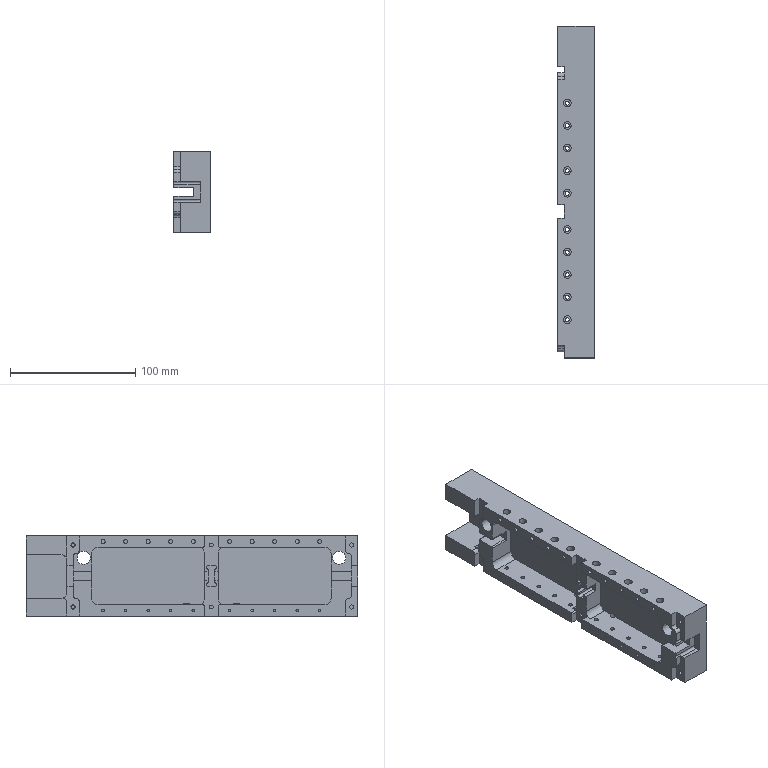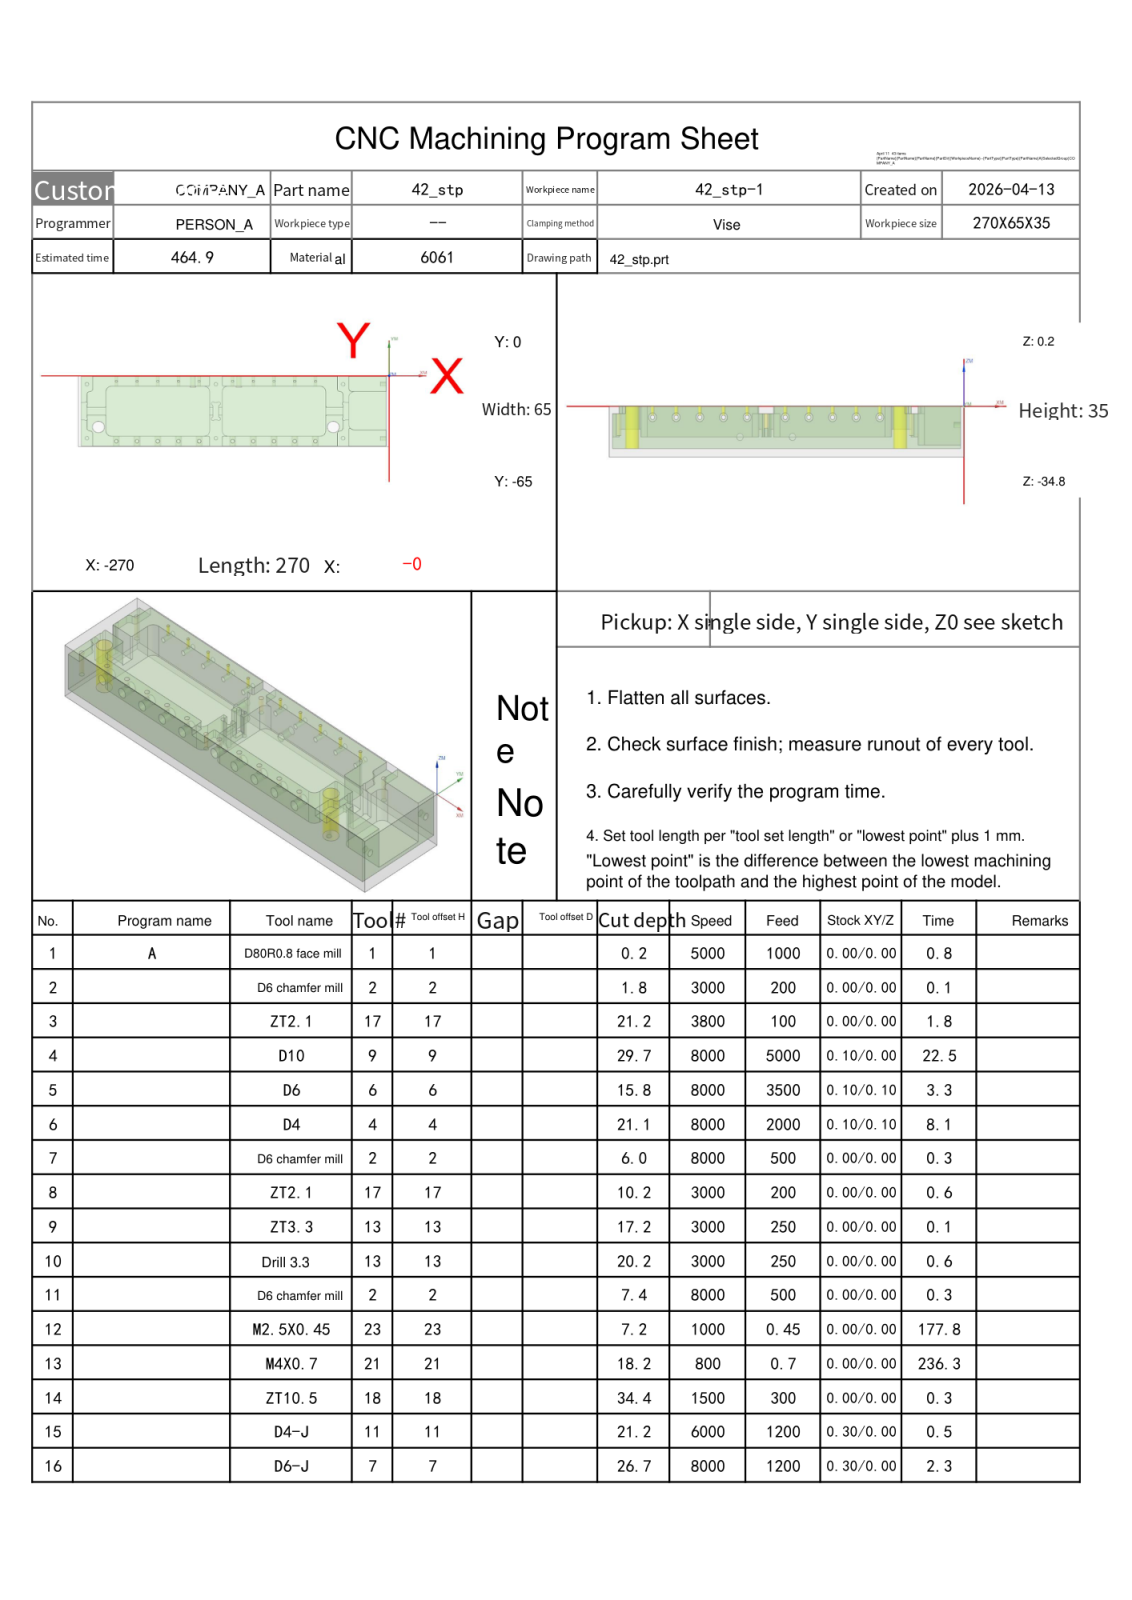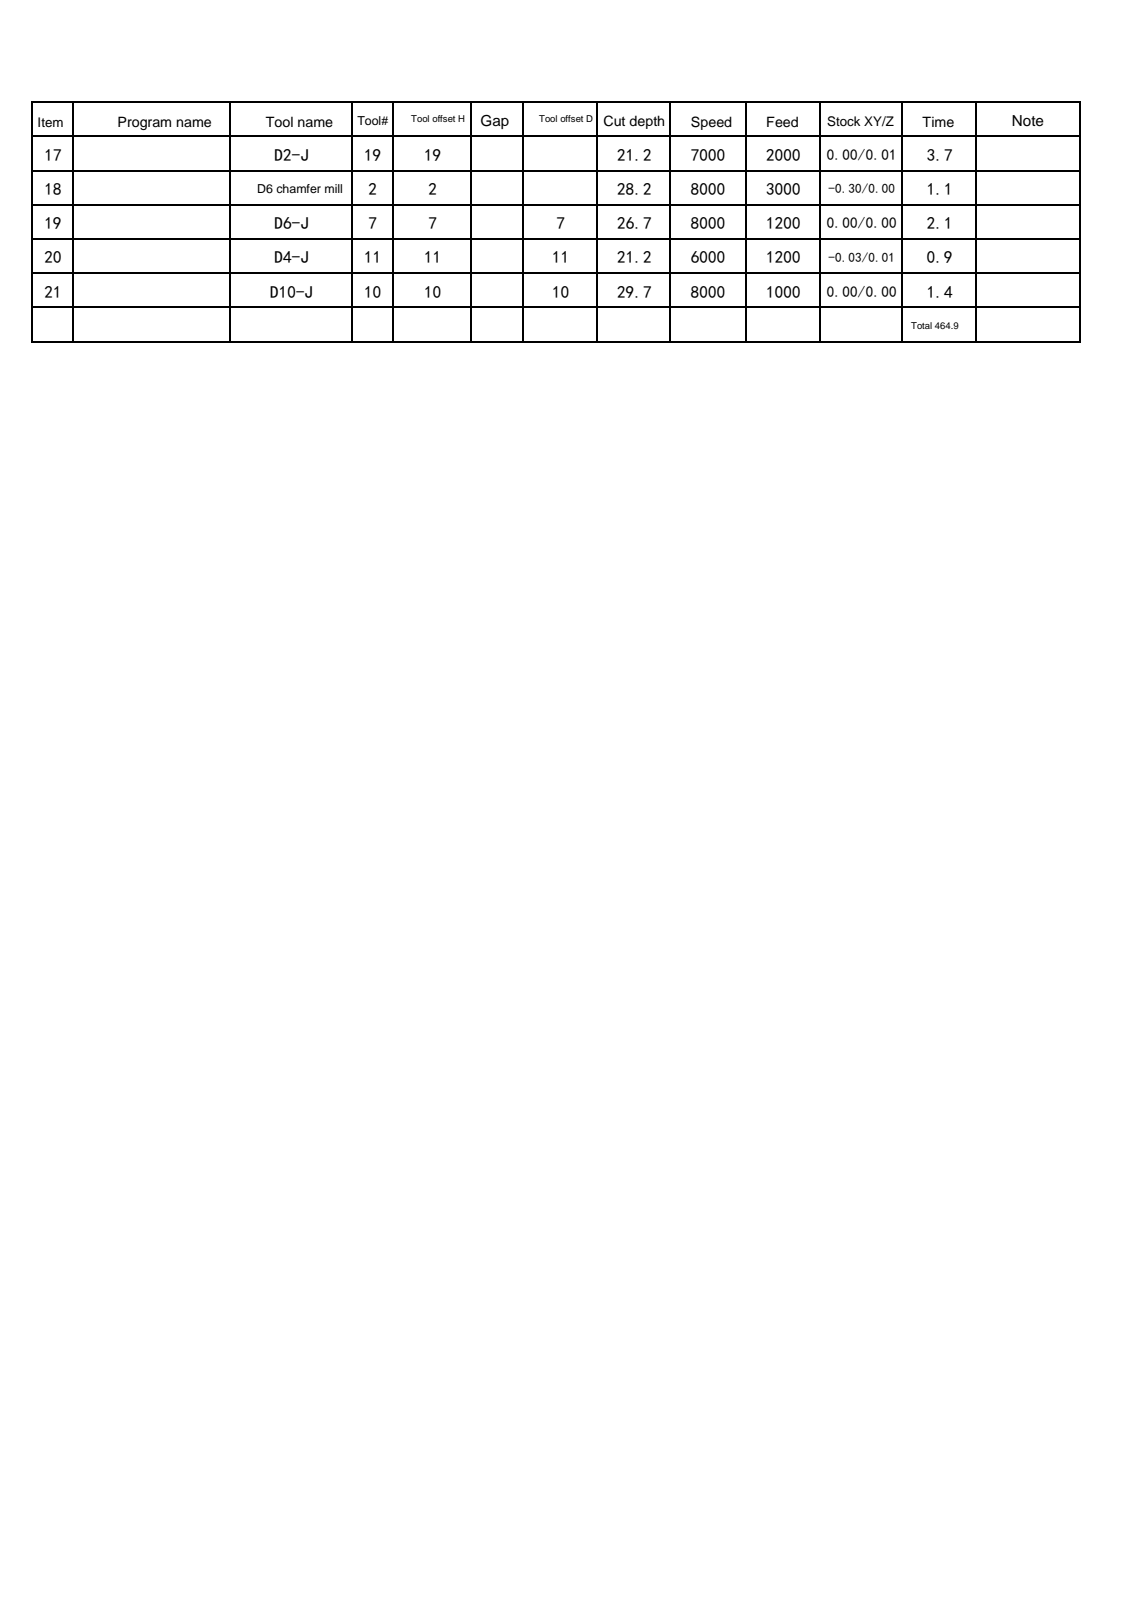NC program | NX | posted by the shop | part box 29 x 265 x 64 mm
Lines 11165 to 11782 of 41846:
N7 T02 M06
(D6 chamfer mill  D=6. R=0. H=02 ce=0.00 di=0.10)
G00 G90 G54 X-48.5 Y-47. M03 S8000
G43 H02 Z20.
M08
G98 G82 X-48.5 Y-47. Z-.8 R1. F500.
X-252.5
G80
G00 Z20.
G00 G90 X-40. Y-7.75 M03 S8000
Z20.
G98 G81 X-40. Y-7.75 Z-5.8 R-4. F500.
X-64. Y-5. Z-.8 R1.
X-82.
X-100.
X-118.
X-136.
X-150.5 Y-7.75 Z-5.8 R-4.
X-165. Y-5. Z-.8 R1.
X-183.
X-201.
X-219.
X-237.
X-262.5 Y-7.75 Z-5.8 R-4.
Y-57.25
X-237. Y-60. Z-.8 R1.
X-219.
X-201.
X-183.
X-165.
X-150.5 Y-57.25 Z-5.8 R-4.
X-136. Y-60. Z-.8 R1.
X-118.
X-100.
X-82.
X-64.
X-40. Y-57.25 Z-5.8 R-4.
G80
G00 Z20.
G00 G90 X-262.5 Y-7.75 M03 S8000
Z20.
G98 G81 X-262.5 Y-7.75 Z-5.8 R-4. F500.
X-237. Y-5. Z-.8 R1.
X-219.
X-201.
X-183.
X-165.
X-150.5 Y-7.75 Z-5.8 R-4.
X-136. Y-5. Z-.8 R1.
X-118.
X-100.
X-82.
X-64.
X-40. Y-7.75 Z-5.8 R-4.
Y-57.25
X-64. Y-60. Z-.8 R1.
X-82.
X-100.
X-118.
X-136.
X-150.5 Y-57.25 Z-5.8 R-4.
X-165. Y-60. Z-.8 R1.
X-183.
X-201.
X-219.
X-237.
X-262.5 Y-57.25 Z-5.8 R-4.
G80
G00 Z20.
G91 G28 Z0.0
M05
M09
G91 G28 Z0.0
M01
N8 T17 M06
(ZT2.1 D=2.1 DR_a=118 H=17)
G00 G90 G54 X-237. Y-5. M03 S3000
G43 H17 Z20.
M08
G98 G83 X-237. Y-5. Z-10. R1. F200. Q2.
X-219.
X-201.
X-183.
X-165.
X-136.
X-118.
X-100.
X-82.
X-64.
G80
G00 Z20.
G91 G28 Z0.0
M05
M09
G91 G28 Z0.0
M01
N9 T13 M06
(ZT3.3 D=3.3 DR_a=118 H=13)
G00 G90 G54 X-150.5 Y-7.75 M03 S3000
G43 H13 Z20.
M08
G98 G83 X-150.5 Y-7.75 Z-17. R-4. F250. Q2.
Y-57.25
G80
G00 Z20.
G91 G28 Z0.0
M05
M09
G91 G28 Z0.0
M01
N10 T13 M06
(Drill 3.3 D=3.3 DR_a=118 H=13)
G00 G90 G54 X-262.5 Y-7.75 M03 S3000
G43 H13 Z20.
M08
G98 G83 X-262.5 Y-7.75 Z-20. R-4. F250. Q2.
Y-57.25
G98 G83 X-237. Y-60. Z-6.926 R1. Q2.
X-219.
X-201.
X-183.
X-165.
X-136.
X-118.
X-100.
X-82.
X-64.
G98 G83 X-40. Y-57.25 Z-20. R-4. Q2.
Y-7.75
G80
G00 Z20.
G91 G28 Z0.0
M05
M09
G91 G28 Z0.0
M01
N11 T02 M06
(D6 chamfer mill  D=6. R=0. H=02 ce=0.00 di=0.10)
G00 G90 G54 X-237. Y-5. M03 S8000
G43 H02 Z20.
M08
G98 G81 X-237. Y-5. Z-1.5 R3. F500.
X-219.
X-201.
X-183.
X-165.
X-136.
X-118.
X-100.
X-82.
X-64.
G80
G00 Z20.
G00 G90 X-150.5 Y-7.75 M03 S8000
Z20.
G98 G81 X-150.5 Y-7.75 Z-7.15 R-2. F500.
Y-57.25
G80
G00 Z20.
G00 G90 X-262.5 Y-7.75 M03 S8000
Z20.
G98 G81 X-262.5 Y-7.75 Z-7.2 R-2. F500.
Y-57.25
X-237. Y-60. Z-2.2 R3.
X-219.
X-201.
X-183.
X-165.
X-136.
X-118.
X-100.
X-82.
X-64.
X-40. Y-57.25 Z-7.2 R-2.
Y-7.75
G80
G00 Z20.
G91 G28 Z0.0
M05
M09
G91 G28 Z0.0
M01
N12 T23 M06
(M2.5X0.45 D=2.05 DR_a=180 H=23)
G00 G90 G54 X-237. Y-5. M03 S1000
G43 H23 Z20.
M08
G95
G98 G84 X-237. Y-5. Z-7. R1. F.45 Q2.
X-219.
X-201.
X-183.
X-165.
X-136.
X-118.
X-100.
X-82.
X-64.
G80
G94
G00 Z20.
G91 G28 Z0.0
M05
M09
G91 G28 Z0.0
M01
N13 T21 M06
(M4X0.7 D=3.3 DR_a=180 H=21)
G00 G90 G54 X-262.5 Y-57.25 M03 S800
G43 H21 Z20.
M08
G95
G98 G84 X-262.5 Y-57.25 Z-18. R1. F.7 Q4.
G98 G84 X-237. Y-60. Z-5.935 R1.
X-219.
X-201.
X-183.
X-165.
X-136.
X-118.
X-100.
X-82.
X-64.
G98 G84 X-40. Y-57.25 Z-18. R1.
Y-7.75
X-262.5
G80
G94
G00 Z20.
G00 G90 X-150.5 Y-57.25 M03 S800
Z20.
G95
G98 G84 X-150.5 Y-57.25 Z-14. R-4. F.7 Q4.
Y-7.75
G80
G94
G00 Z20.
G91 G28 Z0.0
M05
M09
G91 G28 Z0.0
M01
N14 T18 M06
(ZT10.5 D=10.5 DR_a=118 H=18)
G00 G90 G54 X-48.5 Y-47. M03 S1500
G43 H18 Z20.
M08
G98 G83 X-48.5 Y-47. Z-34.155 R1. F300. Q3.
X-252.5
G80
G00 Z20.
G91 G28 Z0.0
M05
M09
G91 G28 Z0.0
M01
N15 T11 M06
(D4-J  D=4. R=0. H=11 ce=0.30 di=0.00)
G00 G90 G54 X-30. Y-32.5 M03 S6000
G43 H11 Z20.
M08
Z-20.5
G01 Z-21. F1200.
X-34.6
Y-38.2
X-37.7
Y-26.8
X-34.6
Y-32.5
Y-33.
X-30.
Z-20.5
G00 Z20.
X-272.5 Y-32.5
Z-20.5
G01 Z-21.
X-267.9
Y-26.8
X-264.8
Y-38.2
X-267.9
Y-32.5
Y-32.
X-272.5
Z-20.5
G00 Z20.
G00 G90 X-40. Y-69.8 M03 S6000
Z20.
Z-4.5
G01 Z-5. F1200.
Y-64.9
X-42.7
Y-53.
G02 X-42.5 Y-52.8 I.2 J0.0
G03 X-37.7 Y-48. I0.0 J4.8
G01 Y-40.618
G03 X-37.759 Y-40.1 I-2.3 J0.0
G01 X-34.6
Y-44.75
G03 X-34.44 Y-45.952 I4.6 J0.0
X-37.3 Y-49.222 I.44 J-3.27
G01 Y-64.9
X-40.
Y-63.1
X-40.9
Y-54.403
G03 X-39.1 Y-53.657 I-1.6 J6.403
G01 Y-63.1
X-40.
X-40.5
Y-69.8
Z-4.5
G00 Z20.
G00 G90 X-40. Y4.8 M03 S6000
Z20.
Z-4.5
G01 Z-5. F1200.
Y-.1
X-37.3
Y-11.5
G03 X-33.546 Y-16.57 I5.3 J0.0
X-34.6 Y-19.5 I3.546 J-2.93
G01 Y-24.9
X-37.759
G03 X-37.7 Y-24.382 I-2.241 J.518
G01 Y-17.
G03 X-42.5 Y-12.2 I-4.8 J0.0
G02 X-42.7 Y-12. I0.0 J.2
G01 Y-.1
X-40.
Y-1.9
X-39.1
Y-11.343
G03 X-40.9 Y-10.597 I-3.4 J-5.657
G01 Y-1.9
X-40.
X-39.5
Y4.8
Z-4.5
G00 Z20.
G00 G90 X-272.5 Y-57.867 M03 S6000
Z20.
Z-4.5
G01 Z-5. F1200.
X-267.9
Y-40.1
X-264.741
G03 X-264.8 Y-40.618 I2.241 J-.518
G01 Y-48.
G03 X-260. Y-52.8 I4.8 J0.0
G02 X-259.8 Y-53. I0.0 J-.2
G01 Y-64.9
X-267.9
Y-57.867
X-265.1
Y-53.635
X-265.831 Y-51.636
X-265.1 Y-53.635
G03 X-262.6 Y-55.141 I5.1 J5.635
G01 Y-62.1
X-265.1
Y-57.867
Y-57.367
X-272.5
Z-4.5
G00 Z20.
Y-7.133
Z-4.5
G01 Z-5.
X-267.9
Y-.1
X-259.8
Y-12.
G02 X-260. Y-12.2 I-.2 J0.0
G03 X-264.8 Y-17. I0.0 J-4.8
G01 Y-24.382
G03 X-264.741 Y-24.9 I2.3 J0.0
G01 X-267.9
Y-7.133
X-265.1
Y-2.9
X-262.6
Y-9.859
G03 X-265.1 Y-11.365 I2.6 J-7.141
G01 X-265.831 Y-13.364
X-265.1 Y-11.365
Y-7.133
Y-6.633
X-272.5
Z-4.5
G00 Z20.
G91 G28 Z0.0
M05
M09
G91 G28 Z0.0
M01
N16 T07 M06
(D6-J  D=6. R=0. H=07 ce=0.30 di=0.00)
G00 G90 G54 X-242.7 Y-14.776 M03 S6000
G43 H07 Z20.
M08
Z-19.5
G01 Y-14.315 Z-19.516 F1200.
X-242.589 Y-13.867 Z-19.532
X-242.361 Y-13.465 Z-19.548
X-242.035 Y-13.139 Z-19.564
X-241.633 Y-12.911 Z-19.581
X-241.185 Y-12.8 Z-19.597
X-201. Z-21.
X-161.
G02 X-159.3 Y-14.5 I0.0 J-1.7
G01 Y-50.5
G02 X-161. Y-52.2 I-1.7 J0.0
G01 X-241.
G02 X-242.7 Y-50.5 I0.0 J1.7
G01 Y-14.5
G02 X-241. Y-12.8 I1.7 J0.0
G01 X-201.
Y-17.
X-163.5
Y-48.
X-238.5
Y-17.
X-201.
Y-21.2
X-167.7
Y-43.8
X-234.3
Y-21.2
X-201.
Y-25.4
X-171.9
Y-39.6
X-230.1
Y-25.4
X-201.
Y-29.6
X-176.1
Y-35.4
X-225.9
Y-29.6
X-201.
Y-32.3
X-178.8
Y-32.7
X-223.2
Y-32.3
X-201.
X-200.5
Y-28.7
Z-20.5
G00 Z20.
X-141.7 Y-14.776
Z-19.5
G01 Y-14.315 Z-19.516
X-141.589 Y-13.867 Z-19.532
X-141.361 Y-13.465 Z-19.548
X-141.035 Y-13.139 Z-19.564
X-140.633 Y-12.911 Z-19.581
X-140.185 Y-12.8 Z-19.597
X-100. Z-21.
X-60.
G02 X-58.3 Y-14.5 I0.0 J-1.7
G01 Y-50.5
G02 X-60. Y-52.2 I-1.7 J0.0
G01 X-140.
G02 X-141.7 Y-50.5 I0.0 J1.7
G01 Y-14.5
G02 X-140. Y-12.8 I1.7 J0.0
G01 X-100.
Y-17.
X-62.5
Y-48.
X-137.5
Y-17.
X-100.
Y-21.2
X-66.7
Y-43.8
X-133.3
Y-21.2
X-100.
Y-25.4
X-70.9
Y-39.6
X-129.1
Y-25.4
X-100.
Y-29.6
X-75.1
Y-35.4
X-124.9
Y-29.6
X-100.
Y-32.3
X-77.8
Y-32.7
X-122.2
Y-32.3
X-100.
X-99.5
Y-28.7
Z-20.5
G00 Z20.
G00 G90 X3.5 Y-32.125 M03 S6000
Z20.
Z-26.
G01 Z-26.5 F1200.
X-1.9
Y-46.45
X-30.
G02 X-31.7 Y-44.75 I0.0 J1.7
G01 Y-19.5
G02 X-30. Y-17.8 I1.7 J0.0
G01 X-1.9
Y-32.125
X-6.1
Y-42.25
X-27.5
Y-22.
X-6.1
Y-32.125
X-10.3
Y-38.05
X-23.3
Y-26.2
X-10.3
Y-32.125
X-14.5
Y-33.85
X-19.1
Y-30.4
X-14.5
Y-32.125
Y-32.625
X-10.9
Z-26.
G00 Z20.
G00 G90 X-160.2 Y-33.7 M03 S8000
Z10.4
Z-3.5
G01 Z-5. F1000.
X-157.8
G03 X-156.6 Y-32.5 I0.0 J1.2
G01 Y-14.5
G03 X-156.763 Y-13.313 I-4.4 J0.0
G01 X-156.776 Y-13.218
G02 X-156.465 Y-12.861 I.36 J0.0
G03 X-152.65 Y-8.5 I-.585 J4.361
G01 Y-.498
G02 X-152.052 Y.1 I.6 J-.002
G01 X-148.948
G02 X-148.35 Y-.498 I-.002 J-.6
G01 Y-8.5
G03 X-144.535 Y-12.861 I4.4 J0.0
G02 X-144.224 Y-13.218 I-.049 J-.357
G01 X-144.237 Y-13.313
G03 X-144.4 Y-14.5 I4.237 J-1.187
G01 Y-50.5
G03 X-144.237 Y-51.687 I4.4 J0.0
G01 X-144.224 Y-51.782
G02 X-144.535 Y-52.139 I-.36 J0.0
G03 X-148.35 Y-56.5 I.585 J-4.361
G01 Y-64.502
G02 X-148.948 Y-65.1 I-.6 J.002
G01 X-152.052
G02 X-152.65 Y-64.502 I.002 J.6
G01 Y-56.5
G03 X-156.465 Y-52.139 I-4.4 J0.0
G02 X-156.776 Y-51.782 I.049 J.357
G01 X-156.763 Y-51.687
G03 X-156.6 Y-50.5 I-4.237 J1.187
G01 Y-29.5
G02 X-156.203 Y-28.935 I.6 J0.0
G01 X-153.997 Y-28.143
G03 X-153.6 Y-27.578 I-.203 J.565
G01 Y-15.397
G02 X-153.306 Y-14.883 I.6 J-.002
G03 X-150.99 Y-12.747 I-3.744 J6.383
G02 X-150.5 Y-12.493 I.49 J-.346
X-150.01 Y-12.747 I0.0 J-.6
G03 X-147.694 Y-14.883 I6.06 J4.247
G02 X-147.4 Y-15.397 I-.306 J-.516
G01 Y-49.603
G02 X-147.694 Y-50.117 I-.6 J.002
G03 X-150.01 Y-52.253 I3.744 J-6.383
G02 X-150.5 Y-52.507 I-.49 J.346
X-150.99 Y-52.253 I0.0 J.6
G03 X-153.306 Y-50.117 I-6.06 J-4.247
G02 X-153.6 Y-49.603 I.306 J.516
G01 Y-31.098
G02 X-153.424 Y-30.674 I.6 J0.0
G01 X-151.076 Y-28.326
G03 X-150.9 Y-27.901 I-.424 J.424
G01 Y-16.685
G02 X-150.765 Y-16.407 I.36 J-.002
G01 X-150.724 Y-16.373
G02 X-150.5 Y-16.295 I.224 J-.282
X-150.276 Y-16.373 I0.0 J-.36
G01 X-150.235 Y-16.407
G02 X-150.1 Y-16.685 I-.225 J-.281
G01 Y-48.315
G02 X-150.235 Y-48.593 I-.36 J.002
G01 X-150.276 Y-48.627
G02 X-150.5 Y-48.705 I-.224 J.282
X-150.724 Y-48.627 I0.0 J.36
G01 X-150.765 Y-48.593
G02 X-150.9 Y-48.315 I.225 J.281
G01 Y-29.5
Y-28.5
G03 X-152.1 Y-27.3 I-1.2 J0.0
G01 Z-3.5
G00 Z10.4
G91 G28 Z0.0
M05
M09
G91 G28 Z0.0
M01